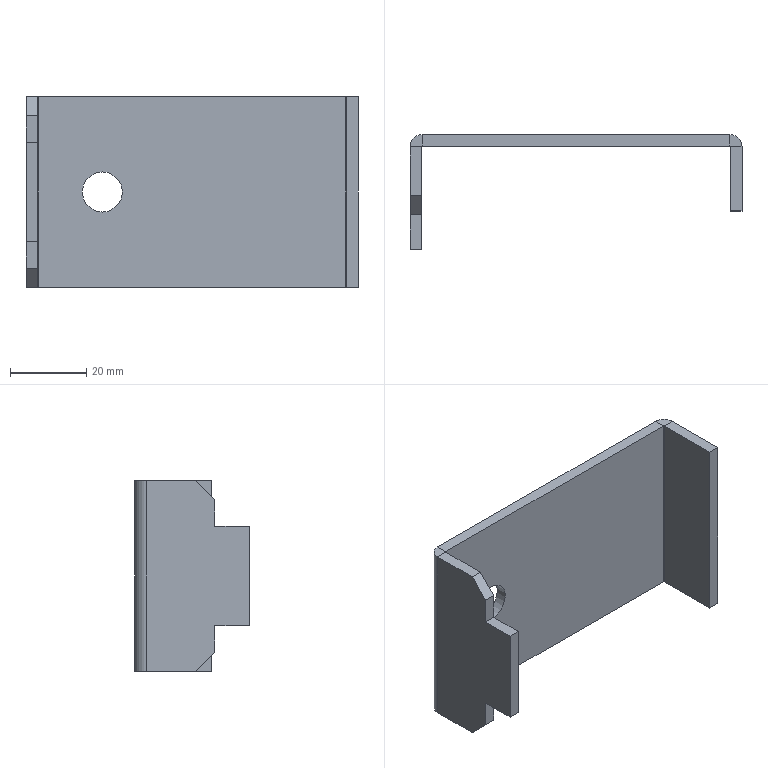Part | SolidWorks | features ICE 4, Chamfer 1, FlatPattern 1, SMBaseFlange 1, SheetMetal 1 | 1 solid | 30 faces | box 87 x 30 x 50 mm | volume 18448 mm3 | plane 24 | cylinder 6 | commonest cylinder face diameters 0.4 x2 6.4 x2 10.5 x2
STEP:
#1=CARTESIAN_POINT('',(-67.,17.,5.25));
#2=VERTEX_POINT('',#1);
#3=CARTESIAN_POINT('',(-67.,17.,-5.25));
#4=VERTEX_POINT('',#3);
#5=CARTESIAN_POINT('',(-67.,17.,0.));
#6=DIRECTION('',(0.,-1.,0.));
#7=DIRECTION('',(1.,0.,0.));
#8=AXIS2_PLACEMENT_3D('',#5,#6,#7);
#9=CIRCLE('',#8,5.25);
#10=EDGE_CURVE('',#2,#4,#9,.T.);
#11=ORIENTED_EDGE('',*,*,#10,.T.);
#12=CARTESIAN_POINT('',(-67.,20.,-5.25));
#13=VERTEX_POINT('',#12);
#14=CARTESIAN_POINT('',(-67.,10.,-5.25));
#15=DIRECTION('',(0.,1.,0.));
#16=VECTOR('',#15,1000.);
#17=LINE('',#14,#16);
#18=EDGE_CURVE('',#4,#13,#17,.T.);
#19=ORIENTED_EDGE('',*,*,#18,.T.);
#20=CARTESIAN_POINT('',(-67.,20.,5.25));
#21=VERTEX_POINT('',#20);
#22=CARTESIAN_POINT('',(-67.,20.,0.));
#23=DIRECTION('',(0.,1.,0.));
#24=DIRECTION('',(0.,0.,1.));
#25=AXIS2_PLACEMENT_3D('',#22,#23,#24);
#26=CIRCLE('',#25,5.25);
#27=EDGE_CURVE('',#13,#21,#26,.T.);
#28=ORIENTED_EDGE('',*,*,#27,.T.);
#29=CARTESIAN_POINT('',(-67.,10.,5.25));
#30=DIRECTION('',(0.,1.,0.));
#31=VECTOR('',#30,1000.);
#32=LINE('',#29,#31);
#33=EDGE_CURVE('',#2,#21,#32,.T.);
#34=ORIENTED_EDGE('',*,*,#33,.F.);
#35=EDGE_LOOP('',(#11,#19,#28,#34));
#36=FACE_OUTER_BOUND('',#35,.T.);
#37=CARTESIAN_POINT('',(-67.,10.,0.));
#38=DIRECTION('',(0.,1.,0.));
#39=DIRECTION('',(0.,0.,1.));
#40=AXIS2_PLACEMENT_3D('',#37,#38,#39);
#41=CYLINDRICAL_SURFACE('',#40,5.25);
#42=ADVANCED_FACE('',(#36),#41,.F.);
#43=CARTESIAN_POINT('',(0.,16.8,25.));
#44=VERTEX_POINT('',#43);
#45=CARTESIAN_POINT('',(-3.,16.8,25.));
#46=VERTEX_POINT('',#45);
#47=CARTESIAN_POINT('',(0.,16.8,25.));
#48=DIRECTION('',(-1.,0.,0.));
#49=VECTOR('',#48,1000.);
#50=LINE('',#47,#49);
#51=EDGE_CURVE('',#44,#46,#50,.T.);
#52=ORIENTED_EDGE('',*,*,#51,.F.);
#53=CARTESIAN_POINT('',(-3.2,20.,25.));
#54=VERTEX_POINT('',#53);
#55=CARTESIAN_POINT('',(-3.2,16.8,25.));
#56=DIRECTION('',(0.,0.,1.));
#57=DIRECTION('',(-1.,0.,0.));
#58=AXIS2_PLACEMENT_3D('',#55,#56,#57);
#59=CIRCLE('',#58,3.2);
#60=EDGE_CURVE('',#44,#54,#59,.T.);
#61=ORIENTED_EDGE('',*,*,#60,.T.);
#62=CARTESIAN_POINT('',(-3.2,17.,25.));
#63=VERTEX_POINT('',#62);
#64=CARTESIAN_POINT('',(-3.2,17.,25.));
#65=DIRECTION('',(0.,1.,0.));
#66=VECTOR('',#65,1000.);
#67=LINE('',#64,#66);
#68=EDGE_CURVE('',#63,#54,#67,.T.);
#69=ORIENTED_EDGE('',*,*,#68,.F.);
#70=CARTESIAN_POINT('',(-3.2,16.8,25.));
#71=DIRECTION('',(0.,0.,1.));
#72=DIRECTION('',(1.,0.,0.));
#73=AXIS2_PLACEMENT_3D('',#70,#71,#72);
#74=CIRCLE('',#73,0.2);
#75=EDGE_CURVE('',#46,#63,#74,.T.);
#76=ORIENTED_EDGE('',*,*,#75,.F.);
#77=EDGE_LOOP('',(#52,#61,#69,#76));
#78=FACE_OUTER_BOUND('',#77,.T.);
#79=CARTESIAN_POINT('',(0.,16.8,25.));
#80=DIRECTION('',(0.,0.,1.));
#81=DIRECTION('',(1.,0.,0.));
#82=AXIS2_PLACEMENT_3D('',#79,#80,#81);
#83=PLANE('',#82);
#84=ADVANCED_FACE('',(#78),#83,.T.);
#85=CARTESIAN_POINT('',(0.,0.,25.));
#86=VERTEX_POINT('',#85);
#87=CARTESIAN_POINT('',(0.,0.,25.));
#88=DIRECTION('',(0.,1.,0.));
#89=VECTOR('',#88,1000.);
#90=LINE('',#87,#89);
#91=EDGE_CURVE('',#86,#44,#90,.T.);
#92=ORIENTED_EDGE('',*,*,#91,.T.);
#93=ORIENTED_EDGE('',*,*,#51,.T.);
#94=CARTESIAN_POINT('',(-3.,0.,25.));
#95=VERTEX_POINT('',#94);
#96=CARTESIAN_POINT('',(-3.,0.,25.));
#97=DIRECTION('',(0.,1.,0.));
#98=VECTOR('',#97,1000.);
#99=LINE('',#96,#98);
#100=EDGE_CURVE('',#95,#46,#99,.T.);
#101=ORIENTED_EDGE('',*,*,#100,.F.);
#102=CARTESIAN_POINT('',(0.,0.,25.));
#103=DIRECTION('',(-1.,0.,0.));
#104=VECTOR('',#103,1000.);
#105=LINE('',#102,#104);
#106=EDGE_CURVE('',#86,#95,#105,.T.);
#107=ORIENTED_EDGE('',*,*,#106,.F.);
#108=EDGE_LOOP('',(#92,#93,#101,#107));
#109=FACE_OUTER_BOUND('',#108,.T.);
#110=CARTESIAN_POINT('',(-3.2,17.,25.));
#111=DIRECTION('',(0.,0.,1.));
#112=DIRECTION('',(1.,0.,0.));
#113=AXIS2_PLACEMENT_3D('',#110,#111,#112);
#114=PLANE('',#113);
#115=ADVANCED_FACE('',(#109),#114,.T.);
#116=CARTESIAN_POINT('',(-3.2,20.,-25.));
#117=VERTEX_POINT('',#116);
#118=CARTESIAN_POINT('',(-3.2,17.,-25.));
#119=VERTEX_POINT('',#118);
#120=CARTESIAN_POINT('',(-3.2,20.,-25.));
#121=DIRECTION('',(0.,-1.,0.));
#122=VECTOR('',#121,1000.);
#123=LINE('',#120,#122);
#124=EDGE_CURVE('',#117,#119,#123,.T.);
#125=ORIENTED_EDGE('',*,*,#124,.F.);
#126=CARTESIAN_POINT('',(0.,16.8,-25.));
#127=VERTEX_POINT('',#126);
#128=CARTESIAN_POINT('',(-3.2,16.8,-25.));
#129=DIRECTION('',(0.,0.,1.));
#130=DIRECTION('',(-1.,0.,0.));
#131=AXIS2_PLACEMENT_3D('',#128,#129,#130);
#132=CIRCLE('',#131,3.2);
#133=EDGE_CURVE('',#127,#117,#132,.T.);
#134=ORIENTED_EDGE('',*,*,#133,.F.);
#135=CARTESIAN_POINT('',(-3.,16.8,-25.));
#136=VERTEX_POINT('',#135);
#137=CARTESIAN_POINT('',(-3.,16.8,-25.));
#138=DIRECTION('',(1.,0.,0.));
#139=VECTOR('',#138,1000.);
#140=LINE('',#137,#139);
#141=EDGE_CURVE('',#136,#127,#140,.T.);
#142=ORIENTED_EDGE('',*,*,#141,.F.);
#143=CARTESIAN_POINT('',(-3.2,16.8,-25.));
#144=DIRECTION('',(0.,0.,1.));
#145=DIRECTION('',(1.,0.,0.));
#146=AXIS2_PLACEMENT_3D('',#143,#144,#145);
#147=CIRCLE('',#146,0.2);
#148=EDGE_CURVE('',#136,#119,#147,.T.);
#149=ORIENTED_EDGE('',*,*,#148,.T.);
#150=EDGE_LOOP('',(#125,#134,#142,#149));
#151=FACE_OUTER_BOUND('',#150,.T.);
#152=CARTESIAN_POINT('',(-3.2,20.,-25.));
#153=DIRECTION('',(0.,0.,-1.));
#154=DIRECTION('',(-1.,0.,0.));
#155=AXIS2_PLACEMENT_3D('',#152,#153,#154);
#156=PLANE('',#155);
#157=ADVANCED_FACE('',(#151),#156,.T.);
#158=CARTESIAN_POINT('',(-83.8,20.,-25.));
#159=VERTEX_POINT('',#158);
#160=CARTESIAN_POINT('',(0.,20.,-25.));
#161=DIRECTION('',(-1.,0.,0.));
#162=VECTOR('',#161,1000.);
#163=LINE('',#160,#162);
#164=EDGE_CURVE('',#117,#159,#163,.T.);
#165=ORIENTED_EDGE('',*,*,#164,.F.);
#166=ORIENTED_EDGE('',*,*,#124,.T.);
#167=CARTESIAN_POINT('',(-83.8,17.,-25.));
#168=VERTEX_POINT('',#167);
#169=CARTESIAN_POINT('',(0.,17.,-25.));
#170=DIRECTION('',(-1.,0.,0.));
#171=VECTOR('',#170,1000.);
#172=LINE('',#169,#171);
#173=EDGE_CURVE('',#119,#168,#172,.T.);
#174=ORIENTED_EDGE('',*,*,#173,.T.);
#175=CARTESIAN_POINT('',(-83.8,17.,-25.));
#176=DIRECTION('',(0.,1.,0.));
#177=VECTOR('',#176,1000.);
#178=LINE('',#175,#177);
#179=EDGE_CURVE('',#168,#159,#178,.T.);
#180=ORIENTED_EDGE('',*,*,#179,.T.);
#181=EDGE_LOOP('',(#165,#166,#174,#180));
#182=FACE_OUTER_BOUND('',#181,.T.);
#183=CARTESIAN_POINT('',(-3.,16.8,-25.));
#184=DIRECTION('',(0.,0.,-1.));
#185=DIRECTION('',(-1.,0.,0.));
#186=AXIS2_PLACEMENT_3D('',#183,#184,#185);
#187=PLANE('',#186);
#188=ADVANCED_FACE('',(#182),#187,.T.);
#189=CARTESIAN_POINT('',(-83.8,20.,25.));
#190=VERTEX_POINT('',#189);
#191=CARTESIAN_POINT('',(-83.8,17.,25.));
#192=VERTEX_POINT('',#191);
#193=CARTESIAN_POINT('',(-83.8,20.,25.));
#194=DIRECTION('',(0.,-1.,0.));
#195=VECTOR('',#194,1000.);
#196=LINE('',#193,#195);
#197=EDGE_CURVE('',#190,#192,#196,.T.);
#198=ORIENTED_EDGE('',*,*,#197,.F.);
#199=CARTESIAN_POINT('',(-87.,16.8,25.));
#200=VERTEX_POINT('',#199);
#201=CARTESIAN_POINT('',(-83.8,16.8,25.));
#202=DIRECTION('',(0.,0.,1.));
#203=DIRECTION('',(-1.,0.,0.));
#204=AXIS2_PLACEMENT_3D('',#201,#202,#203);
#205=CIRCLE('',#204,3.2);
#206=EDGE_CURVE('',#190,#200,#205,.T.);
#207=ORIENTED_EDGE('',*,*,#206,.T.);
#208=CARTESIAN_POINT('',(-84.,16.8,25.));
#209=VERTEX_POINT('',#208);
#210=CARTESIAN_POINT('',(-84.,16.8,25.));
#211=DIRECTION('',(-1.,0.,0.));
#212=VECTOR('',#211,1000.);
#213=LINE('',#210,#212);
#214=EDGE_CURVE('',#209,#200,#213,.T.);
#215=ORIENTED_EDGE('',*,*,#214,.F.);
#216=CARTESIAN_POINT('',(-83.8,16.8,25.));
#217=DIRECTION('',(0.,0.,1.));
#218=DIRECTION('',(1.,0.,0.));
#219=AXIS2_PLACEMENT_3D('',#216,#217,#218);
#220=CIRCLE('',#219,0.2);
#221=EDGE_CURVE('',#192,#209,#220,.T.);
#222=ORIENTED_EDGE('',*,*,#221,.F.);
#223=EDGE_LOOP('',(#198,#207,#215,#222));
#224=FACE_OUTER_BOUND('',#223,.T.);
#225=CARTESIAN_POINT('',(-83.8,20.,25.));
#226=DIRECTION('',(0.,0.,1.));
#227=DIRECTION('',(1.,0.,0.));
#228=AXIS2_PLACEMENT_3D('',#225,#226,#227);
#229=PLANE('',#228);
#230=ADVANCED_FACE('',(#224),#229,.T.);
#231=CARTESIAN_POINT('',(0.,20.,25.));
#232=DIRECTION('',(-1.,0.,0.));
#233=VECTOR('',#232,1000.);
#234=LINE('',#231,#233);
#235=EDGE_CURVE('',#54,#190,#234,.T.);
#236=ORIENTED_EDGE('',*,*,#235,.T.);
#237=ORIENTED_EDGE('',*,*,#197,.T.);
#238=CARTESIAN_POINT('',(0.,17.,25.));
#239=DIRECTION('',(-1.,0.,0.));
#240=VECTOR('',#239,1000.);
#241=LINE('',#238,#240);
#242=EDGE_CURVE('',#63,#192,#241,.T.);
#243=ORIENTED_EDGE('',*,*,#242,.F.);
#244=ORIENTED_EDGE('',*,*,#68,.T.);
#245=EDGE_LOOP('',(#236,#237,#243,#244));
#246=FACE_OUTER_BOUND('',#245,.T.);
#247=CARTESIAN_POINT('',(-84.,16.8,25.));
#248=DIRECTION('',(0.,0.,1.));
#249=DIRECTION('',(1.,0.,0.));
#250=AXIS2_PLACEMENT_3D('',#247,#248,#249);
#251=PLANE('',#250);
#252=ADVANCED_FACE('',(#246),#251,.T.);
#253=CARTESIAN_POINT('',(-87.,16.8,-25.));
#254=VERTEX_POINT('',#253);
#255=CARTESIAN_POINT('',(-84.,16.8,-25.));
#256=VERTEX_POINT('',#255);
#257=CARTESIAN_POINT('',(-87.,16.8,-25.));
#258=DIRECTION('',(1.,0.,0.));
#259=VECTOR('',#258,1000.);
#260=LINE('',#257,#259);
#261=EDGE_CURVE('',#254,#256,#260,.T.);
#262=ORIENTED_EDGE('',*,*,#261,.F.);
#263=CARTESIAN_POINT('',(-83.8,16.8,-25.));
#264=DIRECTION('',(0.,0.,1.));
#265=DIRECTION('',(-1.,0.,0.));
#266=AXIS2_PLACEMENT_3D('',#263,#264,#265);
#267=CIRCLE('',#266,3.2);
#268=EDGE_CURVE('',#159,#254,#267,.T.);
#269=ORIENTED_EDGE('',*,*,#268,.F.);
#270=ORIENTED_EDGE('',*,*,#179,.F.);
#271=CARTESIAN_POINT('',(-83.8,16.8,-25.));
#272=DIRECTION('',(0.,0.,1.));
#273=DIRECTION('',(1.,0.,0.));
#274=AXIS2_PLACEMENT_3D('',#271,#272,#273);
#275=CIRCLE('',#274,0.2);
#276=EDGE_CURVE('',#168,#256,#275,.T.);
#277=ORIENTED_EDGE('',*,*,#276,.T.);
#278=EDGE_LOOP('',(#262,#269,#270,#277));
#279=FACE_OUTER_BOUND('',#278,.T.);
#280=CARTESIAN_POINT('',(-87.,16.8,-25.));
#281=DIRECTION('',(0.,0.,-1.));
#282=DIRECTION('',(-1.,0.,0.));
#283=AXIS2_PLACEMENT_3D('',#280,#281,#282);
#284=PLANE('',#283);
#285=ADVANCED_FACE('',(#279),#284,.T.);
#286=CARTESIAN_POINT('',(-84.,4.,-25.));
#287=VERTEX_POINT('',#286);
#288=CARTESIAN_POINT('',(-84.,20.,-25.));
#289=DIRECTION('',(0.,-1.,0.));
#290=VECTOR('',#289,1000.);
#291=LINE('',#288,#290);
#292=EDGE_CURVE('',#256,#287,#291,.T.);
#293=ORIENTED_EDGE('',*,*,#292,.T.);
#294=CARTESIAN_POINT('',(-87.,4.,-25.));
#295=VERTEX_POINT('',#294);
#296=CARTESIAN_POINT('',(-87.,4.,-25.));
#297=DIRECTION('',(-1.,0.,0.));
#298=VECTOR('',#297,1000.);
#299=LINE('',#296,#298);
#300=EDGE_CURVE('',#287,#295,#299,.T.);
#301=ORIENTED_EDGE('',*,*,#300,.T.);
#302=CARTESIAN_POINT('',(-87.,20.,-25.));
#303=DIRECTION('',(0.,-1.,0.));
#304=VECTOR('',#303,1000.);
#305=LINE('',#302,#304);
#306=EDGE_CURVE('',#254,#295,#305,.T.);
#307=ORIENTED_EDGE('',*,*,#306,.F.);
#308=ORIENTED_EDGE('',*,*,#261,.T.);
#309=EDGE_LOOP('',(#293,#301,#307,#308));
#310=FACE_OUTER_BOUND('',#309,.T.);
#311=CARTESIAN_POINT('',(-83.8,17.,-25.));
#312=DIRECTION('',(0.,0.,-1.));
#313=DIRECTION('',(-1.,0.,0.));
#314=AXIS2_PLACEMENT_3D('',#311,#312,#313);
#315=PLANE('',#314);
#316=ADVANCED_FACE('',(#310),#315,.T.);
#317=ORIENTED_EDGE('',*,*,#306,.T.);
#318=CARTESIAN_POINT('',(-87.,-1.,-20.));
#319=VERTEX_POINT('',#318);
#320=CARTESIAN_POINT('',(-87.,4.,-25.));
#321=DIRECTION('',(0.,-0.7071,0.7071));
#322=VECTOR('',#321,1000.);
#323=LINE('',#320,#322);
#324=EDGE_CURVE('',#295,#319,#323,.T.);
#325=ORIENTED_EDGE('',*,*,#324,.T.);
#326=CARTESIAN_POINT('',(-87.,-1.,-13.));
#327=VERTEX_POINT('',#326);
#328=CARTESIAN_POINT('',(-87.,-1.,-25.));
#329=DIRECTION('',(0.,0.,-1.));
#330=VECTOR('',#329,1000.);
#331=LINE('',#328,#330);
#332=EDGE_CURVE('',#327,#319,#331,.T.);
#333=ORIENTED_EDGE('',*,*,#332,.F.);
#334=CARTESIAN_POINT('',(-87.,-10.,-13.));
#335=VERTEX_POINT('',#334);
#336=CARTESIAN_POINT('',(-87.,-10.,-13.));
#337=DIRECTION('',(0.,1.,0.));
#338=VECTOR('',#337,1000.);
#339=LINE('',#336,#338);
#340=EDGE_CURVE('',#335,#327,#339,.T.);
#341=ORIENTED_EDGE('',*,*,#340,.F.);
#342=CARTESIAN_POINT('',(-87.,-10.,13.));
#343=VERTEX_POINT('',#342);
#344=CARTESIAN_POINT('',(-87.,-10.,25.));
#345=DIRECTION('',(0.,0.,-1.));
#346=VECTOR('',#345,1000.);
#347=LINE('',#344,#346);
#348=EDGE_CURVE('',#343,#335,#347,.T.);
#349=ORIENTED_EDGE('',*,*,#348,.F.);
#350=CARTESIAN_POINT('',(-87.,-1.,13.));
#351=VERTEX_POINT('',#350);
#352=CARTESIAN_POINT('',(-87.,-10.,13.));
#353=DIRECTION('',(0.,-1.,0.));
#354=VECTOR('',#353,1000.);
#355=LINE('',#352,#354);
#356=EDGE_CURVE('',#351,#343,#355,.T.);
#357=ORIENTED_EDGE('',*,*,#356,.F.);
#358=CARTESIAN_POINT('',(-87.,-1.,20.));
#359=VERTEX_POINT('',#358);
#360=CARTESIAN_POINT('',(-87.,-1.,25.));
#361=DIRECTION('',(0.,0.,-1.));
#362=VECTOR('',#361,1000.);
#363=LINE('',#360,#362);
#364=EDGE_CURVE('',#359,#351,#363,.T.);
#365=ORIENTED_EDGE('',*,*,#364,.F.);
#366=CARTESIAN_POINT('',(-87.,4.,25.));
#367=VERTEX_POINT('',#366);
#368=CARTESIAN_POINT('',(-87.,-1.,20.));
#369=DIRECTION('',(0.,0.7071,0.7071));
#370=VECTOR('',#369,1000.);
#371=LINE('',#368,#370);
#372=EDGE_CURVE('',#359,#367,#371,.T.);
#373=ORIENTED_EDGE('',*,*,#372,.T.);
#374=CARTESIAN_POINT('',(-87.,20.,25.));
#375=DIRECTION('',(0.,-1.,0.));
#376=VECTOR('',#375,1000.);
#377=LINE('',#374,#376);
#378=EDGE_CURVE('',#200,#367,#377,.T.);
#379=ORIENTED_EDGE('',*,*,#378,.F.);
#380=CARTESIAN_POINT('',(-87.,16.8,25.));
#381=DIRECTION('',(0.,0.,-1.));
#382=VECTOR('',#381,1000.);
#383=LINE('',#380,#382);
#384=EDGE_CURVE('',#200,#254,#383,.T.);
#385=ORIENTED_EDGE('',*,*,#384,.T.);
#386=EDGE_LOOP('',(#317,#325,#333,#341,#349,#357,#365,#373,#379,#385));
#387=FACE_OUTER_BOUND('',#386,.T.);
#388=CARTESIAN_POINT('',(-87.,20.,25.));
#389=DIRECTION('',(1.,0.,0.));
#390=DIRECTION('',(0.,0.,-1.));
#391=AXIS2_PLACEMENT_3D('',#388,#389,#390);
#392=PLANE('',#391);
#393=ADVANCED_FACE('',(#387),#392,.F.);
#394=CARTESIAN_POINT('',(-84.,-10.,-13.));
#395=VERTEX_POINT('',#394);
#396=CARTESIAN_POINT('',(-77.,-10.,-13.));
#397=DIRECTION('',(-1.,0.,0.));
#398=VECTOR('',#397,1000.);
#399=LINE('',#396,#398);
#400=EDGE_CURVE('',#395,#335,#399,.T.);
#401=ORIENTED_EDGE('',*,*,#400,.F.);
#402=CARTESIAN_POINT('',(-84.,-10.,13.));
#403=VERTEX_POINT('',#402);
#404=CARTESIAN_POINT('',(-84.,-10.,25.));
#405=DIRECTION('',(0.,0.,-1.));
#406=VECTOR('',#405,1000.);
#407=LINE('',#404,#406);
#408=EDGE_CURVE('',#403,#395,#407,.T.);
#409=ORIENTED_EDGE('',*,*,#408,.F.);
#410=CARTESIAN_POINT('',(-77.,-10.,13.));
#411=DIRECTION('',(-1.,0.,0.));
#412=VECTOR('',#411,1000.);
#413=LINE('',#410,#412);
#414=EDGE_CURVE('',#403,#343,#413,.T.);
#415=ORIENTED_EDGE('',*,*,#414,.T.);
#416=ORIENTED_EDGE('',*,*,#348,.T.);
#417=EDGE_LOOP('',(#401,#409,#415,#416));
#418=FACE_OUTER_BOUND('',#417,.T.);
#419=CARTESIAN_POINT('',(-84.,-10.,25.));
#420=DIRECTION('',(0.,-1.,0.));
#421=DIRECTION('',(0.,0.,-1.));
#422=AXIS2_PLACEMENT_3D('',#419,#420,#421);
#423=PLANE('',#422);
#424=ADVANCED_FACE('',(#418),#423,.T.);
#425=CARTESIAN_POINT('',(-84.,-1.,-20.));
#426=VERTEX_POINT('',#425);
#427=CARTESIAN_POINT('',(-84.,-1.,-13.));
#428=VERTEX_POINT('',#427);
#429=CARTESIAN_POINT('',(-84.,-1.,25.));
#430=DIRECTION('',(0.,0.,1.));
#431=VECTOR('',#430,1000.);
#432=LINE('',#429,#431);
#433=EDGE_CURVE('',#426,#428,#432,.T.);
#434=ORIENTED_EDGE('',*,*,#433,.F.);
#435=CARTESIAN_POINT('',(-84.,-13.,-8.));
#436=DIRECTION('',(0.,0.7071,-0.7071));
#437=VECTOR('',#436,1000.);
#438=LINE('',#435,#437);
#439=EDGE_CURVE('',#426,#287,#438,.T.);
#440=ORIENTED_EDGE('',*,*,#439,.T.);
#441=ORIENTED_EDGE('',*,*,#292,.F.);
#442=CARTESIAN_POINT('',(-84.,16.8,25.));
#443=DIRECTION('',(0.,0.,-1.));
#444=VECTOR('',#443,1000.);
#445=LINE('',#442,#444);
#446=EDGE_CURVE('',#209,#256,#445,.T.);
#447=ORIENTED_EDGE('',*,*,#446,.F.);
#448=CARTESIAN_POINT('',(-84.,4.,25.));
#449=VERTEX_POINT('',#448);
#450=CARTESIAN_POINT('',(-84.,20.,25.));
#451=DIRECTION('',(0.,-1.,0.));
#452=VECTOR('',#451,1000.);
#453=LINE('',#450,#452);
#454=EDGE_CURVE('',#209,#449,#453,.T.);
#455=ORIENTED_EDGE('',*,*,#454,.T.);
#456=CARTESIAN_POINT('',(-84.,-1.,20.));
#457=VERTEX_POINT('',#456);
#458=CARTESIAN_POINT('',(-84.,12.,33.));
#459=DIRECTION('',(0.,-0.7071,-0.7071));
#460=VECTOR('',#459,1000.);
#461=LINE('',#458,#460);
#462=EDGE_CURVE('',#449,#457,#461,.T.);
#463=ORIENTED_EDGE('',*,*,#462,.T.);
#464=CARTESIAN_POINT('',(-84.,-1.,13.));
#465=VERTEX_POINT('',#464);
#466=CARTESIAN_POINT('',(-84.,-1.,25.));
#467=DIRECTION('',(0.,0.,1.));
#468=VECTOR('',#467,1000.);
#469=LINE('',#466,#468);
#470=EDGE_CURVE('',#465,#457,#469,.T.);
#471=ORIENTED_EDGE('',*,*,#470,.F.);
#472=CARTESIAN_POINT('',(-84.,20.,13.));
#473=DIRECTION('',(0.,1.,0.));
#474=VECTOR('',#473,1000.);
#475=LINE('',#472,#474);
#476=EDGE_CURVE('',#403,#465,#475,.T.);
#477=ORIENTED_EDGE('',*,*,#476,.F.);
#478=ORIENTED_EDGE('',*,*,#408,.T.);
#479=CARTESIAN_POINT('',(-84.,20.,-13.));
#480=DIRECTION('',(0.,-1.,0.));
#481=VECTOR('',#480,1000.);
#482=LINE('',#479,#481);
#483=EDGE_CURVE('',#428,#395,#482,.T.);
#484=ORIENTED_EDGE('',*,*,#483,.F.);
#485=EDGE_LOOP('',(#434,#440,#441,#447,#455,#463,#471,#477,#478,#484));
#486=FACE_OUTER_BOUND('',#485,.T.);
#487=CARTESIAN_POINT('',(-84.,20.,25.));
#488=DIRECTION('',(1.,0.,0.));
#489=DIRECTION('',(0.,0.,-1.));
#490=AXIS2_PLACEMENT_3D('',#487,#488,#489);
#491=PLANE('',#490);
#492=ADVANCED_FACE('',(#486),#491,.T.);
#493=ORIENTED_EDGE('',*,*,#276,.F.);
#494=CARTESIAN_POINT('',(-83.8,17.,25.));
#495=DIRECTION('',(0.,0.,-1.));
#496=VECTOR('',#495,1000.);
#497=LINE('',#494,#496);
#498=EDGE_CURVE('',#192,#168,#497,.T.);
#499=ORIENTED_EDGE('',*,*,#498,.F.);
#500=ORIENTED_EDGE('',*,*,#221,.T.);
#501=ORIENTED_EDGE('',*,*,#446,.T.);
#502=EDGE_LOOP('',(#493,#499,#500,#501));
#503=FACE_OUTER_BOUND('',#502,.T.);
#504=CARTESIAN_POINT('',(-83.8,16.8,25.));
#505=DIRECTION('',(0.,0.,-1.));
#506=DIRECTION('',(-1.,0.,0.));
#507=AXIS2_PLACEMENT_3D('',#504,#505,#506);
#508=CYLINDRICAL_SURFACE('',#507,0.2);
#509=ADVANCED_FACE('',(#503),#508,.F.);
#510=ORIENTED_EDGE('',*,*,#10,.F.);
#511=CARTESIAN_POINT('',(-67.,17.,0.));
#512=DIRECTION('',(0.,-1.,0.));
#513=DIRECTION('',(1.,0.,0.));
#514=AXIS2_PLACEMENT_3D('',#511,#512,#513);
#515=CIRCLE('',#514,5.25);
#516=EDGE_CURVE('',#4,#2,#515,.T.);
#517=ORIENTED_EDGE('',*,*,#516,.F.);
#518=EDGE_LOOP('',(#510,#517));
#519=FACE_BOUND('',#518,.T.);
#520=ORIENTED_EDGE('',*,*,#173,.F.);
#521=CARTESIAN_POINT('',(-3.2,17.,25.));
#522=DIRECTION('',(0.,0.,-1.));
#523=VECTOR('',#522,1000.);
#524=LINE('',#521,#523);
#525=EDGE_CURVE('',#63,#119,#524,.T.);
#526=ORIENTED_EDGE('',*,*,#525,.F.);
#527=ORIENTED_EDGE('',*,*,#242,.T.);
#528=ORIENTED_EDGE('',*,*,#498,.T.);
#529=EDGE_LOOP('',(#520,#526,#527,#528));
#530=FACE_OUTER_BOUND('',#529,.T.);
#531=CARTESIAN_POINT('',(0.,17.,25.));
#532=DIRECTION('',(0.,-1.,0.));
#533=DIRECTION('',(1.,0.,0.));
#534=AXIS2_PLACEMENT_3D('',#531,#532,#533);
#535=PLANE('',#534);
#536=ADVANCED_FACE('',(#519,#530),#535,.T.);
#537=ORIENTED_EDGE('',*,*,#148,.F.);
#538=CARTESIAN_POINT('',(-3.,16.8,25.));
#539=DIRECTION('',(0.,0.,-1.));
#540=VECTOR('',#539,1000.);
#541=LINE('',#538,#540);
#542=EDGE_CURVE('',#46,#136,#541,.T.);
#543=ORIENTED_EDGE('',*,*,#542,.F.);
#544=ORIENTED_EDGE('',*,*,#75,.T.);
#545=ORIENTED_EDGE('',*,*,#525,.T.);
#546=EDGE_LOOP('',(#537,#543,#544,#545));
#547=FACE_OUTER_BOUND('',#546,.T.);
#548=CARTESIAN_POINT('',(-3.2,16.8,25.));
#549=DIRECTION('',(0.,0.,-1.));
#550=DIRECTION('',(-1.,0.,0.));
#551=AXIS2_PLACEMENT_3D('',#548,#549,#550);
#552=CYLINDRICAL_SURFACE('',#551,0.2);
#553=ADVANCED_FACE('',(#547),#552,.F.);
#554=CARTESIAN_POINT('',(-3.,0.,-25.));
#555=VERTEX_POINT('',#554);
#556=CARTESIAN_POINT('',(-3.,0.,-25.));
#557=DIRECTION('',(0.,1.,0.));
#558=VECTOR('',#557,1000.);
#559=LINE('',#556,#558);
#560=EDGE_CURVE('',#555,#136,#559,.T.);
#561=ORIENTED_EDGE('',*,*,#560,.F.);
#562=CARTESIAN_POINT('',(-3.,0.,25.));
#563=DIRECTION('',(0.,0.,-1.));
#564=VECTOR('',#563,1000.);
#565=LINE('',#562,#564);
#566=EDGE_CURVE('',#95,#555,#565,.T.);
#567=ORIENTED_EDGE('',*,*,#566,.F.);
#568=ORIENTED_EDGE('',*,*,#100,.T.);
#569=ORIENTED_EDGE('',*,*,#542,.T.);
#570=EDGE_LOOP('',(#561,#567,#568,#569));
#571=FACE_OUTER_BOUND('',#570,.T.);
#572=CARTESIAN_POINT('',(-3.,0.,25.));
#573=DIRECTION('',(-1.,0.,0.));
#574=DIRECTION('',(0.,0.,1.));
#575=AXIS2_PLACEMENT_3D('',#572,#573,#574);
#576=PLANE('',#575);
#577=ADVANCED_FACE('',(#571),#576,.T.);
#578=CARTESIAN_POINT('',(0.,0.,-25.));
#579=VERTEX_POINT('',#578);
#580=CARTESIAN_POINT('',(0.,0.,-25.));
#581=DIRECTION('',(-1.,0.,0.));
#582=VECTOR('',#581,1000.);
#583=LINE('',#580,#582);
#584=EDGE_CURVE('',#579,#555,#583,.T.);
#585=ORIENTED_EDGE('',*,*,#584,.F.);
#586=CARTESIAN_POINT('',(0.,0.,25.));
#587=DIRECTION('',(0.,0.,-1.));
#588=VECTOR('',#587,1000.);
#589=LINE('',#586,#588);
#590=EDGE_CURVE('',#86,#579,#589,.T.);
#591=ORIENTED_EDGE('',*,*,#590,.F.);
#592=ORIENTED_EDGE('',*,*,#106,.T.);
#593=ORIENTED_EDGE('',*,*,#566,.T.);
#594=EDGE_LOOP('',(#585,#591,#592,#593));
#595=FACE_OUTER_BOUND('',#594,.T.);
#596=CARTESIAN_POINT('',(0.,0.,25.));
#597=DIRECTION('',(0.,-1.,0.));
#598=DIRECTION('',(0.,0.,-1.));
#599=AXIS2_PLACEMENT_3D('',#596,#597,#598);
#600=PLANE('',#599);
#601=ADVANCED_FACE('',(#595),#600,.T.);
#602=CARTESIAN_POINT('',(0.,0.,-25.));
#603=DIRECTION('',(0.,1.,0.));
#604=VECTOR('',#603,1000.);
#605=LINE('',#602,#604);
#606=EDGE_CURVE('',#579,#127,#605,.T.);
#607=ORIENTED_EDGE('',*,*,#606,.T.);
#608=CARTESIAN_POINT('',(0.,16.8,25.));
#609=DIRECTION('',(0.,0.,-1.));
#610=VECTOR('',#609,1000.);
#611=LINE('',#608,#610);
#612=EDGE_CURVE('',#44,#127,#611,.T.);
#613=ORIENTED_EDGE('',*,*,#612,.F.);
#614=ORIENTED_EDGE('',*,*,#91,.F.);
#615=ORIENTED_EDGE('',*,*,#590,.T.);
#616=EDGE_LOOP('',(#607,#613,#614,#615));
#617=FACE_OUTER_BOUND('',#616,.T.);
#618=CARTESIAN_POINT('',(0.,0.,25.));
#619=DIRECTION('',(-1.,0.,0.));
#620=DIRECTION('',(0.,0.,1.));
#621=AXIS2_PLACEMENT_3D('',#618,#619,#620);
#622=PLANE('',#621);
#623=ADVANCED_FACE('',(#617),#622,.F.);
#624=ORIENTED_EDGE('',*,*,#133,.T.);
#625=CARTESIAN_POINT('',(-3.2,20.,25.));
#626=DIRECTION('',(0.,0.,-1.));
#627=VECTOR('',#626,1000.);
#628=LINE('',#625,#627);
#629=EDGE_CURVE('',#54,#117,#628,.T.);
#630=ORIENTED_EDGE('',*,*,#629,.F.);
#631=ORIENTED_EDGE('',*,*,#60,.F.);
#632=ORIENTED_EDGE('',*,*,#612,.T.);
#633=EDGE_LOOP('',(#624,#630,#631,#632));
#634=FACE_OUTER_BOUND('',#633,.T.);
#635=CARTESIAN_POINT('',(-3.2,16.8,25.));
#636=DIRECTION('',(0.,0.,-1.));
#637=DIRECTION('',(-1.,0.,0.));
#638=AXIS2_PLACEMENT_3D('',#635,#636,#637);
#639=CYLINDRICAL_SURFACE('',#638,3.2);
#640=ADVANCED_FACE('',(#634),#639,.T.);
#641=CARTESIAN_POINT('',(-67.,20.,0.));
#642=DIRECTION('',(0.,1.,0.));
#643=DIRECTION('',(0.,0.,1.));
#644=AXIS2_PLACEMENT_3D('',#641,#642,#643);
#645=CIRCLE('',#644,5.25);
#646=EDGE_CURVE('',#21,#13,#645,.T.);
#647=ORIENTED_EDGE('',*,*,#646,.F.);
#648=ORIENTED_EDGE('',*,*,#27,.F.);
#649=EDGE_LOOP('',(#647,#648));
#650=FACE_BOUND('',#649,.T.);
#651=ORIENTED_EDGE('',*,*,#164,.T.);
#652=CARTESIAN_POINT('',(-83.8,20.,25.));
#653=DIRECTION('',(0.,0.,-1.));
#654=VECTOR('',#653,1000.);
#655=LINE('',#652,#654);
#656=EDGE_CURVE('',#190,#159,#655,.T.);
#657=ORIENTED_EDGE('',*,*,#656,.F.);
#658=ORIENTED_EDGE('',*,*,#235,.F.);
#659=ORIENTED_EDGE('',*,*,#629,.T.);
#660=EDGE_LOOP('',(#651,#657,#658,#659));
#661=FACE_OUTER_BOUND('',#660,.T.);
#662=CARTESIAN_POINT('',(0.,20.,25.));
#663=DIRECTION('',(0.,-1.,0.));
#664=DIRECTION('',(1.,0.,0.));
#665=AXIS2_PLACEMENT_3D('',#662,#663,#664);
#666=PLANE('',#665);
#667=ADVANCED_FACE('',(#650,#661),#666,.F.);
#668=ORIENTED_EDGE('',*,*,#268,.T.);
#669=ORIENTED_EDGE('',*,*,#384,.F.);
#670=ORIENTED_EDGE('',*,*,#206,.F.);
#671=ORIENTED_EDGE('',*,*,#656,.T.);
#672=EDGE_LOOP('',(#668,#669,#670,#671));
#673=FACE_OUTER_BOUND('',#672,.T.);
#674=CARTESIAN_POINT('',(-83.8,16.8,25.));
#675=DIRECTION('',(0.,0.,-1.));
#676=DIRECTION('',(-1.,0.,0.));
#677=AXIS2_PLACEMENT_3D('',#674,#675,#676);
#678=CYLINDRICAL_SURFACE('',#677,3.2);
#679=ADVANCED_FACE('',(#673),#678,.T.);
#680=ORIENTED_EDGE('',*,*,#378,.T.);
#681=CARTESIAN_POINT('',(-84.,4.,25.));
#682=DIRECTION('',(1.,0.,0.));
#683=VECTOR('',#682,1000.);
#684=LINE('',#681,#683);
#685=EDGE_CURVE('',#367,#449,#684,.T.);
#686=ORIENTED_EDGE('',*,*,#685,.T.);
#687=ORIENTED_EDGE('',*,*,#454,.F.);
#688=ORIENTED_EDGE('',*,*,#214,.T.);
#689=EDGE_LOOP('',(#680,#686,#687,#688));
#690=FACE_OUTER_BOUND('',#689,.T.);
#691=CARTESIAN_POINT('',(-83.8,16.8,25.));
#692=DIRECTION('',(0.,0.,1.));
#693=DIRECTION('',(1.,0.,0.));
#694=AXIS2_PLACEMENT_3D('',#691,#692,#693);
#695=PLANE('',#694);
#696=ADVANCED_FACE('',(#690),#695,.T.);
#697=ORIENTED_EDGE('',*,*,#560,.T.);
#698=ORIENTED_EDGE('',*,*,#141,.T.);
#699=ORIENTED_EDGE('',*,*,#606,.F.);
#700=ORIENTED_EDGE('',*,*,#584,.T.);
#701=EDGE_LOOP('',(#697,#698,#699,#700));
#702=FACE_OUTER_BOUND('',#701,.T.);
#703=CARTESIAN_POINT('',(-83.8,16.8,-25.));
#704=DIRECTION('',(0.,0.,1.));
#705=DIRECTION('',(1.,0.,0.));
#706=AXIS2_PLACEMENT_3D('',#703,#704,#705);
#707=PLANE('',#706);
#708=ADVANCED_FACE('',(#702),#707,.F.);
#709=ORIENTED_EDGE('',*,*,#18,.F.);
#710=ORIENTED_EDGE('',*,*,#516,.T.);
#711=ORIENTED_EDGE('',*,*,#33,.T.);
#712=ORIENTED_EDGE('',*,*,#646,.T.);
#713=EDGE_LOOP('',(#709,#710,#711,#712));
#714=FACE_OUTER_BOUND('',#713,.T.);
#715=CARTESIAN_POINT('',(-67.,10.,0.));
#716=DIRECTION('',(0.,1.,0.));
#717=DIRECTION('',(0.,0.,1.));
#718=AXIS2_PLACEMENT_3D('',#715,#716,#717);
#719=CYLINDRICAL_SURFACE('',#718,5.25);
#720=ADVANCED_FACE('',(#714),#719,.F.);
#721=ORIENTED_EDGE('',*,*,#476,.T.);
#722=CARTESIAN_POINT('',(-77.,-1.,13.));
#723=DIRECTION('',(-1.,0.,0.));
#724=VECTOR('',#723,1000.);
#725=LINE('',#722,#724);
#726=EDGE_CURVE('',#465,#351,#725,.T.);
#727=ORIENTED_EDGE('',*,*,#726,.T.);
#728=ORIENTED_EDGE('',*,*,#356,.T.);
#729=ORIENTED_EDGE('',*,*,#414,.F.);
#730=EDGE_LOOP('',(#721,#727,#728,#729));
#731=FACE_OUTER_BOUND('',#730,.T.);
#732=CARTESIAN_POINT('',(-77.,-10.,13.));
#733=DIRECTION('',(0.,0.,-1.));
#734=DIRECTION('',(-1.,0.,0.));
#735=AXIS2_PLACEMENT_3D('',#732,#733,#734);
#736=PLANE('',#735);
#737=ADVANCED_FACE('',(#731),#736,.F.);
#738=ORIENTED_EDGE('',*,*,#470,.T.);
#739=CARTESIAN_POINT('',(-87.,-1.,20.));
#740=DIRECTION('',(-1.,0.,0.));
#741=VECTOR('',#740,1000.);
#742=LINE('',#739,#741);
#743=EDGE_CURVE('',#457,#359,#742,.T.);
#744=ORIENTED_EDGE('',*,*,#743,.T.);
#745=ORIENTED_EDGE('',*,*,#364,.T.);
#746=ORIENTED_EDGE('',*,*,#726,.F.);
#747=EDGE_LOOP('',(#738,#744,#745,#746));
#748=FACE_OUTER_BOUND('',#747,.T.);
#749=CARTESIAN_POINT('',(-77.,-1.,25.));
#750=DIRECTION('',(0.,1.,0.));
#751=DIRECTION('',(0.,0.,1.));
#752=AXIS2_PLACEMENT_3D('',#749,#750,#751);
#753=PLANE('',#752);
#754=ADVANCED_FACE('',(#748),#753,.F.);
#755=ORIENTED_EDGE('',*,*,#332,.T.);
#756=CARTESIAN_POINT('',(-84.,-1.,-20.));
#757=DIRECTION('',(1.,0.,0.));
#758=VECTOR('',#757,1000.);
#759=LINE('',#756,#758);
#760=EDGE_CURVE('',#319,#426,#759,.T.);
#761=ORIENTED_EDGE('',*,*,#760,.T.);
#762=ORIENTED_EDGE('',*,*,#433,.T.);
#763=CARTESIAN_POINT('',(-77.,-1.,-13.));
#764=DIRECTION('',(-1.,0.,0.));
#765=VECTOR('',#764,1000.);
#766=LINE('',#763,#765);
#767=EDGE_CURVE('',#428,#327,#766,.T.);
#768=ORIENTED_EDGE('',*,*,#767,.T.);
#769=EDGE_LOOP('',(#755,#761,#762,#768));
#770=FACE_OUTER_BOUND('',#769,.T.);
#771=CARTESIAN_POINT('',(-77.,-1.,-25.));
#772=DIRECTION('',(0.,1.,0.));
#773=DIRECTION('',(0.,0.,1.));
#774=AXIS2_PLACEMENT_3D('',#771,#772,#773);
#775=PLANE('',#774);
#776=ADVANCED_FACE('',(#770),#775,.F.);
#777=ORIENTED_EDGE('',*,*,#483,.T.);
#778=ORIENTED_EDGE('',*,*,#400,.T.);
#779=ORIENTED_EDGE('',*,*,#340,.T.);
#780=ORIENTED_EDGE('',*,*,#767,.F.);
#781=EDGE_LOOP('',(#777,#778,#779,#780));
#782=FACE_OUTER_BOUND('',#781,.T.);
#783=CARTESIAN_POINT('',(-77.,-10.,-13.));
#784=DIRECTION('',(0.,0.,1.));
#785=DIRECTION('',(1.,0.,0.));
#786=AXIS2_PLACEMENT_3D('',#783,#784,#785);
#787=PLANE('',#786);
#788=ADVANCED_FACE('',(#782),#787,.F.);
#789=ORIENTED_EDGE('',*,*,#439,.F.);
#790=ORIENTED_EDGE('',*,*,#760,.F.);
#791=ORIENTED_EDGE('',*,*,#324,.F.);
#792=ORIENTED_EDGE('',*,*,#300,.F.);
#793=EDGE_LOOP('',(#789,#790,#791,#792));
#794=FACE_OUTER_BOUND('',#793,.T.);
#795=CARTESIAN_POINT('',(-83.8,4.,-25.));
#796=DIRECTION('',(0.,-0.7071,-0.7071));
#797=DIRECTION('',(1.,0.,0.));
#798=AXIS2_PLACEMENT_3D('',#795,#796,#797);
#799=PLANE('',#798);
#800=ADVANCED_FACE('',(#794),#799,.T.);
#801=ORIENTED_EDGE('',*,*,#462,.F.);
#802=ORIENTED_EDGE('',*,*,#685,.F.);
#803=ORIENTED_EDGE('',*,*,#372,.F.);
#804=ORIENTED_EDGE('',*,*,#743,.F.);
#805=EDGE_LOOP('',(#801,#802,#803,#804));
#806=FACE_OUTER_BOUND('',#805,.T.);
#807=CARTESIAN_POINT('',(-77.,-1.,20.));
#808=DIRECTION('',(0.,-0.7071,0.7071));
#809=DIRECTION('',(1.,0.,0.));
#810=AXIS2_PLACEMENT_3D('',#807,#808,#809);
#811=PLANE('',#810);
#812=ADVANCED_FACE('',(#806),#811,.T.);
#813=CLOSED_SHELL('',(#42,#84,#115,#157,#188,#230,#252,#285,#316,#393,#424,#492,#509,#536,#553,#577,#601,#623,#640,#667,#679,#696,#708,#720,#737,#754,#776,#788,#800,#812));
#814=MANIFOLD_SOLID_BREP('',#813);
#815=CARTESIAN_POINT('',(0.,0.,0.));
#816=DIRECTION('',(0.,0.,1.));
#817=DIRECTION('',(1.,0.,0.));
#818=AXIS2_PLACEMENT_3D('',#815,#816,#817);
#819=(LENGTH_UNIT()NAMED_UNIT(*)SI_UNIT(.MILLI.,.METRE.));
#820=UNCERTAINTY_MEASURE_WITH_UNIT(LENGTH_MEASURE(0.00001),#819,'','');
#821=(NAMED_UNIT(*)PLANE_ANGLE_UNIT()SI_UNIT($,.RADIAN.));
#822=(NAMED_UNIT(*)SI_UNIT($,.STERADIAN.)SOLID_ANGLE_UNIT());
#823=(GEOMETRIC_REPRESENTATION_CONTEXT(3)GLOBAL_UNCERTAINTY_ASSIGNED_CONTEXT((#820))GLOBAL_UNIT_ASSIGNED_CONTEXT((#819,#821,#822))REPRESENTATION_CONTEXT('',''));
#824=ADVANCED_BREP_SHAPE_REPRESENTATION('',(#814,#818),#823);